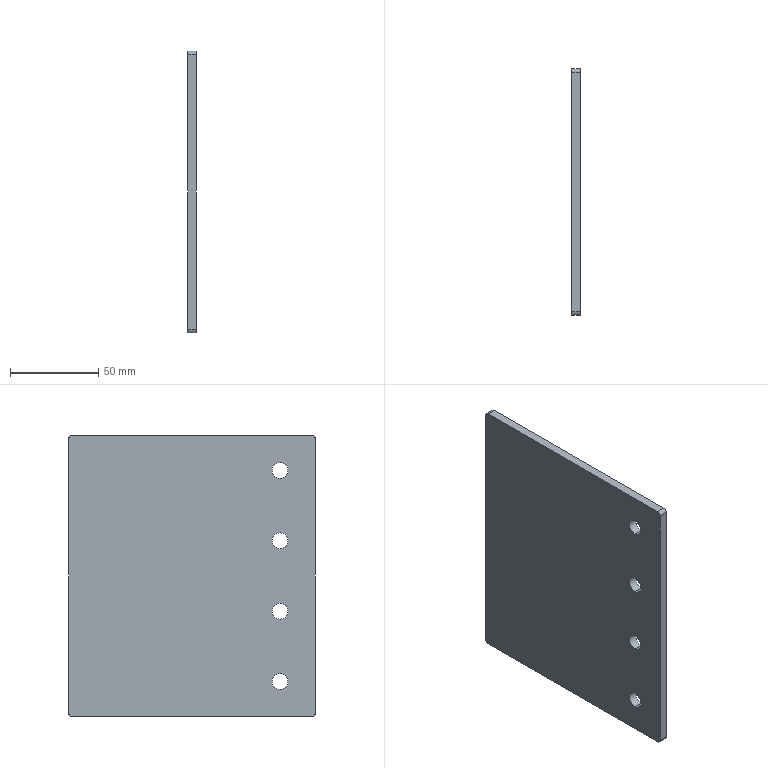Part | STEP file | 1 solid | 18 faces | box 5 x 140 x 160 mm | volume 110710 mm3 | cylinder 12 | plane 6 | commonest cylinder face diameters 9 x8 4 x4